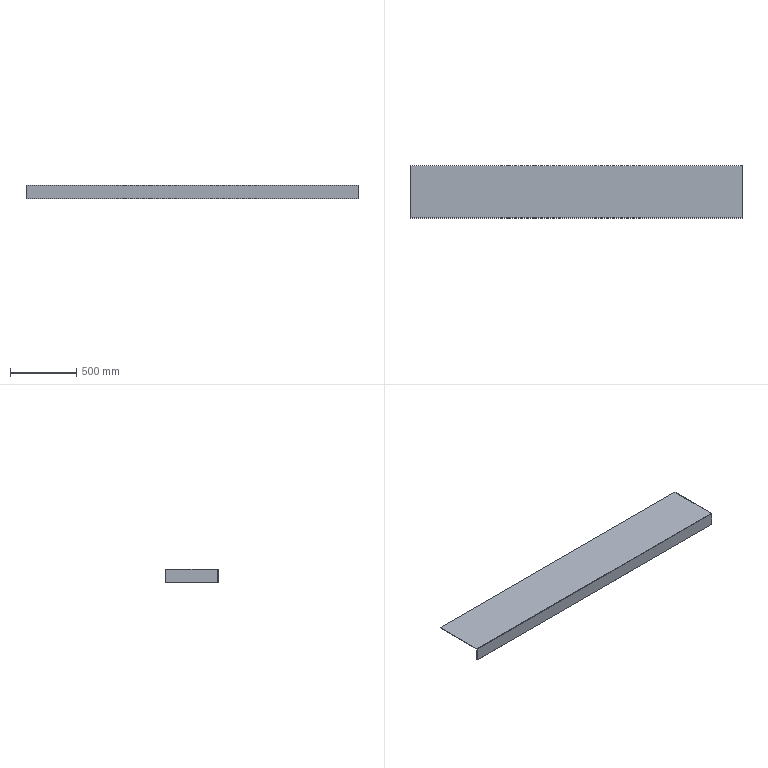Part | STEP file | PN_0035 third-floor site mounting plate 1_Default<As Machined> | 2 solids | 14 faces | box 2515 x 394 x 103 mm | volume 3844530 mm3 | plane 14
STEP:
#1=CARTESIAN_POINT('',(0.,0.,0.));
#2=DIRECTION('',(0.,0.,1.));
#3=DIRECTION('',(1.,0.,0.));
#4=AXIS2_PLACEMENT_3D('',#1,#2,#3);
#5=CARTESIAN_POINT('',(1257.5,-197.,0.));
#6=VERTEX_POINT('',#5);
#7=CARTESIAN_POINT('',(1257.5,197.,0.));
#8=VERTEX_POINT('',#7);
#9=CARTESIAN_POINT('',(1257.5,197.,0.));
#10=DIRECTION('',(0.,1.,0.));
#11=VECTOR('',#10,1.);
#12=LINE('',#9,#11);
#13=CARTESIAN_POINT('',(1257.5,197.,-3.));
#14=DIRECTION('',(1.,0.,0.));
#15=DIRECTION('',(0.,0.,-1.));
#16=AXIS2_PLACEMENT_3D('',#13,#14,#15);
#17=PLANE('',#16);
#18=CARTESIAN_POINT('',(-3.,0.));
#19=DIRECTION('',(0.,1.));
#20=VECTOR('',#19,1.);
#21=LINE('',#18,#20);
#22=(GEOMETRIC_REPRESENTATION_CONTEXT(2)PARAMETRIC_REPRESENTATION_CONTEXT()REPRESENTATION_CONTEXT('',''));
#23=DEFINITIONAL_REPRESENTATION('',(#21),#22);
#24=PCURVE('',#17,#23);
#25=CARTESIAN_POINT('',(0.,0.,0.));
#26=DIRECTION('',(0.,0.,1.));
#27=DIRECTION('',(1.,0.,0.));
#28=AXIS2_PLACEMENT_3D('',#25,#26,#27);
#29=PLANE('',#28);
#30=CARTESIAN_POINT('',(1257.5,197.));
#31=DIRECTION('',(0.,1.));
#32=VECTOR('',#31,1.);
#33=LINE('',#30,#32);
#34=(GEOMETRIC_REPRESENTATION_CONTEXT(2)PARAMETRIC_REPRESENTATION_CONTEXT()REPRESENTATION_CONTEXT('',''));
#35=DEFINITIONAL_REPRESENTATION('',(#33),#34);
#36=PCURVE('',#29,#35);
#37=SURFACE_CURVE('',#12,(#24,#36),.PCURVE_S1.);
#38=EDGE_CURVE('',#6,#8,#37,.T.);
#39=ORIENTED_EDGE('',*,*,#38,.F.);
#40=CARTESIAN_POINT('',(1257.5,-197.,-3.));
#41=VERTEX_POINT('',#40);
#42=CARTESIAN_POINT('',(1257.5,-197.,-3.));
#43=DIRECTION('',(0.,0.,1.));
#44=VECTOR('',#43,1.);
#45=LINE('',#42,#44);
#46=CARTESIAN_POINT('',(0.,-394.));
#47=DIRECTION('',(-1.,0.));
#48=VECTOR('',#47,1.);
#49=LINE('',#46,#48);
#50=(GEOMETRIC_REPRESENTATION_CONTEXT(2)PARAMETRIC_REPRESENTATION_CONTEXT()REPRESENTATION_CONTEXT('',''));
#51=DEFINITIONAL_REPRESENTATION('',(#49),#50);
#52=PCURVE('',#17,#51);
#53=CARTESIAN_POINT('',(-1257.5,-197.,-3.));
#54=DIRECTION('',(0.,-1.,0.));
#55=DIRECTION('',(0.,0.,-1.));
#56=AXIS2_PLACEMENT_3D('',#53,#54,#55);
#57=PLANE('',#56);
#58=CARTESIAN_POINT('',(0.,2515.));
#59=DIRECTION('',(-1.,0.));
#60=VECTOR('',#59,1.);
#61=LINE('',#58,#60);
#62=(GEOMETRIC_REPRESENTATION_CONTEXT(2)PARAMETRIC_REPRESENTATION_CONTEXT()REPRESENTATION_CONTEXT('',''));
#63=DEFINITIONAL_REPRESENTATION('',(#61),#62);
#64=PCURVE('',#57,#63);
#65=SURFACE_CURVE('',#45,(#52,#64),.PCURVE_S1.);
#66=EDGE_CURVE('',#41,#6,#65,.T.);
#67=ORIENTED_EDGE('',*,*,#66,.F.);
#68=CARTESIAN_POINT('',(1257.5,197.,-3.));
#69=VERTEX_POINT('',#68);
#70=CARTESIAN_POINT('',(1257.5,197.,-3.));
#71=DIRECTION('',(0.,1.,0.));
#72=VECTOR('',#71,1.);
#73=LINE('',#70,#72);
#74=CARTESIAN_POINT('',(0.,0.));
#75=DIRECTION('',(0.,1.));
#76=VECTOR('',#75,1.);
#77=LINE('',#74,#76);
#78=(GEOMETRIC_REPRESENTATION_CONTEXT(2)PARAMETRIC_REPRESENTATION_CONTEXT()REPRESENTATION_CONTEXT('',''));
#79=DEFINITIONAL_REPRESENTATION('',(#77),#78);
#80=PCURVE('',#17,#79);
#81=CARTESIAN_POINT('',(0.,0.,-3.));
#82=DIRECTION('',(0.,0.,1.));
#83=DIRECTION('',(1.,0.,0.));
#84=AXIS2_PLACEMENT_3D('',#81,#82,#83);
#85=PLANE('',#84);
#86=CARTESIAN_POINT('',(1257.5,197.));
#87=DIRECTION('',(0.,1.));
#88=VECTOR('',#87,1.);
#89=LINE('',#86,#88);
#90=(GEOMETRIC_REPRESENTATION_CONTEXT(2)PARAMETRIC_REPRESENTATION_CONTEXT()REPRESENTATION_CONTEXT('',''));
#91=DEFINITIONAL_REPRESENTATION('',(#89),#90);
#92=PCURVE('',#85,#91);
#93=SURFACE_CURVE('',#73,(#80,#92),.PCURVE_S1.);
#94=EDGE_CURVE('',#41,#69,#93,.T.);
#95=ORIENTED_EDGE('',*,*,#94,.T.);
#96=CARTESIAN_POINT('',(1257.5,197.,-3.));
#97=DIRECTION('',(0.,0.,1.));
#98=VECTOR('',#97,1.);
#99=LINE('',#96,#98);
#100=CARTESIAN_POINT('',(0.,0.));
#101=DIRECTION('',(-1.,0.));
#102=VECTOR('',#101,1.);
#103=LINE('',#100,#102);
#104=(GEOMETRIC_REPRESENTATION_CONTEXT(2)PARAMETRIC_REPRESENTATION_CONTEXT()REPRESENTATION_CONTEXT('',''));
#105=DEFINITIONAL_REPRESENTATION('',(#103),#104);
#106=PCURVE('',#17,#105);
#107=CARTESIAN_POINT('',(-1257.5,197.,-3.));
#108=DIRECTION('',(0.,1.,0.));
#109=DIRECTION('',(0.,0.,1.));
#110=AXIS2_PLACEMENT_3D('',#107,#108,#109);
#111=PLANE('',#110);
#112=CARTESIAN_POINT('',(0.,2515.));
#113=DIRECTION('',(1.,0.));
#114=VECTOR('',#113,1.);
#115=LINE('',#112,#114);
#116=(GEOMETRIC_REPRESENTATION_CONTEXT(2)PARAMETRIC_REPRESENTATION_CONTEXT()REPRESENTATION_CONTEXT('',''));
#117=DEFINITIONAL_REPRESENTATION('',(#115),#116);
#118=PCURVE('',#111,#117);
#119=SURFACE_CURVE('',#99,(#106,#118),.PCURVE_S1.);
#120=EDGE_CURVE('',#69,#8,#119,.T.);
#121=ORIENTED_EDGE('',*,*,#120,.T.);
#122=EDGE_LOOP('',(#39,#67,#95,#121));
#123=FACE_BOUND('',#122,.T.);
#124=ADVANCED_FACE('',(#123),#17,.T.);
#125=CARTESIAN_POINT('',(-1257.5,-197.,0.));
#126=VERTEX_POINT('',#125);
#127=CARTESIAN_POINT('',(-1257.5,-197.,0.));
#128=DIRECTION('',(1.,0.,0.));
#129=VECTOR('',#128,1.);
#130=LINE('',#127,#129);
#131=CARTESIAN_POINT('',(-3.,0.));
#132=DIRECTION('',(0.,1.));
#133=VECTOR('',#132,1.);
#134=LINE('',#131,#133);
#135=(GEOMETRIC_REPRESENTATION_CONTEXT(2)PARAMETRIC_REPRESENTATION_CONTEXT()REPRESENTATION_CONTEXT('',''));
#136=DEFINITIONAL_REPRESENTATION('',(#134),#135);
#137=PCURVE('',#57,#136);
#138=CARTESIAN_POINT('',(-1257.5,-197.));
#139=DIRECTION('',(1.,0.));
#140=VECTOR('',#139,1.);
#141=LINE('',#138,#140);
#142=(GEOMETRIC_REPRESENTATION_CONTEXT(2)PARAMETRIC_REPRESENTATION_CONTEXT()REPRESENTATION_CONTEXT('',''));
#143=DEFINITIONAL_REPRESENTATION('',(#141),#142);
#144=PCURVE('',#29,#143);
#145=SURFACE_CURVE('',#130,(#137,#144),.PCURVE_S1.);
#146=EDGE_CURVE('',#126,#6,#145,.T.);
#147=ORIENTED_EDGE('',*,*,#146,.F.);
#148=CARTESIAN_POINT('',(-1257.5,-197.,-3.));
#149=VERTEX_POINT('',#148);
#150=CARTESIAN_POINT('',(-1257.5,-197.,-3.));
#151=DIRECTION('',(0.,0.,1.));
#152=VECTOR('',#151,1.);
#153=LINE('',#150,#152);
#154=CARTESIAN_POINT('',(0.,0.));
#155=DIRECTION('',(-1.,0.));
#156=VECTOR('',#155,1.);
#157=LINE('',#154,#156);
#158=(GEOMETRIC_REPRESENTATION_CONTEXT(2)PARAMETRIC_REPRESENTATION_CONTEXT()REPRESENTATION_CONTEXT('',''));
#159=DEFINITIONAL_REPRESENTATION('',(#157),#158);
#160=PCURVE('',#57,#159);
#161=CARTESIAN_POINT('',(-1257.5,197.,-3.));
#162=DIRECTION('',(-1.,0.,0.));
#163=DIRECTION('',(0.,0.,1.));
#164=AXIS2_PLACEMENT_3D('',#161,#162,#163);
#165=PLANE('',#164);
#166=CARTESIAN_POINT('',(0.,-394.));
#167=DIRECTION('',(1.,0.));
#168=VECTOR('',#167,1.);
#169=LINE('',#166,#168);
#170=(GEOMETRIC_REPRESENTATION_CONTEXT(2)PARAMETRIC_REPRESENTATION_CONTEXT()REPRESENTATION_CONTEXT('',''));
#171=DEFINITIONAL_REPRESENTATION('',(#169),#170);
#172=PCURVE('',#165,#171);
#173=SURFACE_CURVE('',#153,(#160,#172),.PCURVE_S1.);
#174=EDGE_CURVE('',#149,#126,#173,.T.);
#175=ORIENTED_EDGE('',*,*,#174,.F.);
#176=CARTESIAN_POINT('',(-1257.5,-197.,-3.));
#177=DIRECTION('',(1.,0.,0.));
#178=VECTOR('',#177,1.);
#179=LINE('',#176,#178);
#180=CARTESIAN_POINT('',(0.,0.));
#181=DIRECTION('',(0.,1.));
#182=VECTOR('',#181,1.);
#183=LINE('',#180,#182);
#184=(GEOMETRIC_REPRESENTATION_CONTEXT(2)PARAMETRIC_REPRESENTATION_CONTEXT()REPRESENTATION_CONTEXT('',''));
#185=DEFINITIONAL_REPRESENTATION('',(#183),#184);
#186=PCURVE('',#57,#185);
#187=CARTESIAN_POINT('',(-1257.5,-197.));
#188=DIRECTION('',(1.,0.));
#189=VECTOR('',#188,1.);
#190=LINE('',#187,#189);
#191=(GEOMETRIC_REPRESENTATION_CONTEXT(2)PARAMETRIC_REPRESENTATION_CONTEXT()REPRESENTATION_CONTEXT('',''));
#192=DEFINITIONAL_REPRESENTATION('',(#190),#191);
#193=PCURVE('',#85,#192);
#194=SURFACE_CURVE('',#179,(#186,#193),.PCURVE_S1.);
#195=EDGE_CURVE('',#149,#41,#194,.T.);
#196=ORIENTED_EDGE('',*,*,#195,.T.);
#197=ORIENTED_EDGE('',*,*,#66,.T.);
#198=EDGE_LOOP('',(#147,#175,#196,#197));
#199=FACE_BOUND('',#198,.T.);
#200=ADVANCED_FACE('',(#199),#57,.T.);
#201=CARTESIAN_POINT('',(-1257.5,197.,0.));
#202=VERTEX_POINT('',#201);
#203=CARTESIAN_POINT('',(-1257.5,197.,0.));
#204=DIRECTION('',(0.,-1.,0.));
#205=VECTOR('',#204,1.);
#206=LINE('',#203,#205);
#207=CARTESIAN_POINT('',(3.,0.));
#208=DIRECTION('',(0.,-1.));
#209=VECTOR('',#208,1.);
#210=LINE('',#207,#209);
#211=(GEOMETRIC_REPRESENTATION_CONTEXT(2)PARAMETRIC_REPRESENTATION_CONTEXT()REPRESENTATION_CONTEXT('',''));
#212=DEFINITIONAL_REPRESENTATION('',(#210),#211);
#213=PCURVE('',#165,#212);
#214=CARTESIAN_POINT('',(-1257.5,197.));
#215=DIRECTION('',(0.,-1.));
#216=VECTOR('',#215,1.);
#217=LINE('',#214,#216);
#218=(GEOMETRIC_REPRESENTATION_CONTEXT(2)PARAMETRIC_REPRESENTATION_CONTEXT()REPRESENTATION_CONTEXT('',''));
#219=DEFINITIONAL_REPRESENTATION('',(#217),#218);
#220=PCURVE('',#29,#219);
#221=SURFACE_CURVE('',#206,(#213,#220),.PCURVE_S1.);
#222=EDGE_CURVE('',#202,#126,#221,.T.);
#223=ORIENTED_EDGE('',*,*,#222,.F.);
#224=CARTESIAN_POINT('',(-1257.5,197.,-3.));
#225=VERTEX_POINT('',#224);
#226=CARTESIAN_POINT('',(-1257.5,197.,-3.));
#227=DIRECTION('',(0.,0.,1.));
#228=VECTOR('',#227,1.);
#229=LINE('',#226,#228);
#230=CARTESIAN_POINT('',(0.,0.));
#231=DIRECTION('',(1.,0.));
#232=VECTOR('',#231,1.);
#233=LINE('',#230,#232);
#234=(GEOMETRIC_REPRESENTATION_CONTEXT(2)PARAMETRIC_REPRESENTATION_CONTEXT()REPRESENTATION_CONTEXT('',''));
#235=DEFINITIONAL_REPRESENTATION('',(#233),#234);
#236=PCURVE('',#165,#235);
#237=CARTESIAN_POINT('',(0.,0.));
#238=DIRECTION('',(1.,0.));
#239=VECTOR('',#238,1.);
#240=LINE('',#237,#239);
#241=(GEOMETRIC_REPRESENTATION_CONTEXT(2)PARAMETRIC_REPRESENTATION_CONTEXT()REPRESENTATION_CONTEXT('',''));
#242=DEFINITIONAL_REPRESENTATION('',(#240),#241);
#243=PCURVE('',#111,#242);
#244=SURFACE_CURVE('',#229,(#236,#243),.PCURVE_S1.);
#245=EDGE_CURVE('',#225,#202,#244,.T.);
#246=ORIENTED_EDGE('',*,*,#245,.F.);
#247=CARTESIAN_POINT('',(-1257.5,197.,-3.));
#248=DIRECTION('',(0.,-1.,0.));
#249=VECTOR('',#248,1.);
#250=LINE('',#247,#249);
#251=CARTESIAN_POINT('',(0.,0.));
#252=DIRECTION('',(0.,-1.));
#253=VECTOR('',#252,1.);
#254=LINE('',#251,#253);
#255=(GEOMETRIC_REPRESENTATION_CONTEXT(2)PARAMETRIC_REPRESENTATION_CONTEXT()REPRESENTATION_CONTEXT('',''));
#256=DEFINITIONAL_REPRESENTATION('',(#254),#255);
#257=PCURVE('',#165,#256);
#258=CARTESIAN_POINT('',(-1257.5,197.));
#259=DIRECTION('',(0.,-1.));
#260=VECTOR('',#259,1.);
#261=LINE('',#258,#260);
#262=(GEOMETRIC_REPRESENTATION_CONTEXT(2)PARAMETRIC_REPRESENTATION_CONTEXT()REPRESENTATION_CONTEXT('',''));
#263=DEFINITIONAL_REPRESENTATION('',(#261),#262);
#264=PCURVE('',#85,#263);
#265=SURFACE_CURVE('',#250,(#257,#264),.PCURVE_S1.);
#266=EDGE_CURVE('',#225,#149,#265,.T.);
#267=ORIENTED_EDGE('',*,*,#266,.T.);
#268=ORIENTED_EDGE('',*,*,#174,.T.);
#269=EDGE_LOOP('',(#223,#246,#267,#268));
#270=FACE_BOUND('',#269,.T.);
#271=ADVANCED_FACE('',(#270),#165,.T.);
#272=CARTESIAN_POINT('',(-1257.5,197.,0.));
#273=DIRECTION('',(-1.,0.,0.));
#274=VECTOR('',#273,1.);
#275=LINE('',#272,#274);
#276=CARTESIAN_POINT('',(3.,0.));
#277=DIRECTION('',(0.,-1.));
#278=VECTOR('',#277,1.);
#279=LINE('',#276,#278);
#280=(GEOMETRIC_REPRESENTATION_CONTEXT(2)PARAMETRIC_REPRESENTATION_CONTEXT()REPRESENTATION_CONTEXT('',''));
#281=DEFINITIONAL_REPRESENTATION('',(#279),#280);
#282=PCURVE('',#111,#281);
#283=CARTESIAN_POINT('',(-1257.5,197.));
#284=DIRECTION('',(-1.,0.));
#285=VECTOR('',#284,1.);
#286=LINE('',#283,#285);
#287=(GEOMETRIC_REPRESENTATION_CONTEXT(2)PARAMETRIC_REPRESENTATION_CONTEXT()REPRESENTATION_CONTEXT('',''));
#288=DEFINITIONAL_REPRESENTATION('',(#286),#287);
#289=PCURVE('',#29,#288);
#290=SURFACE_CURVE('',#275,(#282,#289),.PCURVE_S1.);
#291=EDGE_CURVE('',#8,#202,#290,.T.);
#292=ORIENTED_EDGE('',*,*,#291,.F.);
#293=ORIENTED_EDGE('',*,*,#120,.F.);
#294=CARTESIAN_POINT('',(-1257.5,197.,-3.));
#295=DIRECTION('',(-1.,0.,0.));
#296=VECTOR('',#295,1.);
#297=LINE('',#294,#296);
#298=CARTESIAN_POINT('',(0.,0.));
#299=DIRECTION('',(0.,-1.));
#300=VECTOR('',#299,1.);
#301=LINE('',#298,#300);
#302=(GEOMETRIC_REPRESENTATION_CONTEXT(2)PARAMETRIC_REPRESENTATION_CONTEXT()REPRESENTATION_CONTEXT('',''));
#303=DEFINITIONAL_REPRESENTATION('',(#301),#302);
#304=PCURVE('',#111,#303);
#305=CARTESIAN_POINT('',(-1257.5,197.));
#306=DIRECTION('',(-1.,0.));
#307=VECTOR('',#306,1.);
#308=LINE('',#305,#307);
#309=(GEOMETRIC_REPRESENTATION_CONTEXT(2)PARAMETRIC_REPRESENTATION_CONTEXT()REPRESENTATION_CONTEXT('',''));
#310=DEFINITIONAL_REPRESENTATION('',(#308),#309);
#311=PCURVE('',#85,#310);
#312=SURFACE_CURVE('',#297,(#304,#311),.PCURVE_S1.);
#313=EDGE_CURVE('',#69,#225,#312,.T.);
#314=ORIENTED_EDGE('',*,*,#313,.T.);
#315=ORIENTED_EDGE('',*,*,#245,.T.);
#316=EDGE_LOOP('',(#292,#293,#314,#315));
#317=FACE_BOUND('',#316,.T.);
#318=ADVANCED_FACE('',(#317),#111,.T.);
#319=ORIENTED_EDGE('',*,*,#94,.F.);
#320=ORIENTED_EDGE('',*,*,#195,.F.);
#321=ORIENTED_EDGE('',*,*,#266,.F.);
#322=ORIENTED_EDGE('',*,*,#313,.F.);
#323=EDGE_LOOP('',(#319,#320,#321,#322));
#324=FACE_BOUND('',#323,.T.);
#325=ADVANCED_FACE('',(#324),#85,.F.);
#326=ORIENTED_EDGE('',*,*,#38,.T.);
#327=ORIENTED_EDGE('',*,*,#291,.T.);
#328=ORIENTED_EDGE('',*,*,#222,.T.);
#329=ORIENTED_EDGE('',*,*,#146,.T.);
#330=EDGE_LOOP('',(#326,#327,#328,#329));
#331=FACE_BOUND('',#330,.T.);
#332=ADVANCED_FACE('',(#331),#29,.T.);
#333=CLOSED_SHELL('',(#124,#200,#271,#318,#325,#332));
#334=MANIFOLD_SOLID_BREP('',#333);
#335=CARTESIAN_POINT('',(1254.5,-194.,-3.));
#336=VERTEX_POINT('',#335);
#337=CARTESIAN_POINT('',(1254.5,197.,-3.));
#338=VERTEX_POINT('',#337);
#339=CARTESIAN_POINT('',(1254.5,-197.,-3.));
#340=DIRECTION('',(0.,1.,0.));
#341=VECTOR('',#340,1.);
#342=LINE('',#339,#341);
#343=CARTESIAN_POINT('',(1254.5,-197.,-103.));
#344=DIRECTION('',(1.,0.,0.));
#345=DIRECTION('',(0.,0.,-1.));
#346=AXIS2_PLACEMENT_3D('',#343,#344,#345);
#347=PLANE('',#346);
#348=CARTESIAN_POINT('',(-100.,0.));
#349=DIRECTION('',(0.,1.));
#350=VECTOR('',#349,1.);
#351=LINE('',#348,#350);
#352=(GEOMETRIC_REPRESENTATION_CONTEXT(2)PARAMETRIC_REPRESENTATION_CONTEXT()REPRESENTATION_CONTEXT('',''));
#353=DEFINITIONAL_REPRESENTATION('',(#351),#352);
#354=PCURVE('',#347,#353);
#355=CARTESIAN_POINT('',(0.,0.,-3.));
#356=DIRECTION('',(0.,0.,1.));
#357=DIRECTION('',(1.,0.,0.));
#358=AXIS2_PLACEMENT_3D('',#355,#356,#357);
#359=PLANE('',#358);
#360=CARTESIAN_POINT('',(1254.5,-197.));
#361=DIRECTION('',(0.,1.));
#362=VECTOR('',#361,1.);
#363=LINE('',#360,#362);
#364=(GEOMETRIC_REPRESENTATION_CONTEXT(2)PARAMETRIC_REPRESENTATION_CONTEXT()REPRESENTATION_CONTEXT('',''));
#365=DEFINITIONAL_REPRESENTATION('',(#363),#364);
#366=PCURVE('',#359,#365);
#367=SURFACE_CURVE('',#342,(#354,#366),.PCURVE_S1.);
#368=EDGE_CURVE('',#336,#338,#367,.T.);
#369=ORIENTED_EDGE('',*,*,#368,.T.);
#370=CARTESIAN_POINT('',(1254.5,197.,-103.));
#371=VERTEX_POINT('',#370);
#372=CARTESIAN_POINT('',(1254.5,197.,-103.));
#373=DIRECTION('',(0.,0.,1.));
#374=VECTOR('',#373,1.);
#375=LINE('',#372,#374);
#376=CARTESIAN_POINT('',(0.,394.));
#377=DIRECTION('',(-1.,0.));
#378=VECTOR('',#377,1.);
#379=LINE('',#376,#378);
#380=(GEOMETRIC_REPRESENTATION_CONTEXT(2)PARAMETRIC_REPRESENTATION_CONTEXT()REPRESENTATION_CONTEXT('',''));
#381=DEFINITIONAL_REPRESENTATION('',(#379),#380);
#382=PCURVE('',#347,#381);
#383=CARTESIAN_POINT('',(1257.5,197.,-103.));
#384=DIRECTION('',(0.,1.,0.));
#385=DIRECTION('',(0.,0.,1.));
#386=AXIS2_PLACEMENT_3D('',#383,#384,#385);
#387=PLANE('',#386);
#388=CARTESIAN_POINT('',(0.,-3.));
#389=DIRECTION('',(1.,0.));
#390=VECTOR('',#389,1.);
#391=LINE('',#388,#390);
#392=(GEOMETRIC_REPRESENTATION_CONTEXT(2)PARAMETRIC_REPRESENTATION_CONTEXT()REPRESENTATION_CONTEXT('',''));
#393=DEFINITIONAL_REPRESENTATION('',(#391),#392);
#394=PCURVE('',#387,#393);
#395=SURFACE_CURVE('',#375,(#382,#394),.PCURVE_S1.);
#396=EDGE_CURVE('',#371,#338,#395,.T.);
#397=ORIENTED_EDGE('',*,*,#396,.F.);
#398=CARTESIAN_POINT('',(1254.5,-194.,-103.));
#399=VERTEX_POINT('',#398);
#400=CARTESIAN_POINT('',(1254.5,-197.,-103.));
#401=DIRECTION('',(0.,1.,0.));
#402=VECTOR('',#401,1.);
#403=LINE('',#400,#402);
#404=CARTESIAN_POINT('',(0.,0.));
#405=DIRECTION('',(0.,1.));
#406=VECTOR('',#405,1.);
#407=LINE('',#404,#406);
#408=(GEOMETRIC_REPRESENTATION_CONTEXT(2)PARAMETRIC_REPRESENTATION_CONTEXT()REPRESENTATION_CONTEXT('',''));
#409=DEFINITIONAL_REPRESENTATION('',(#407),#408);
#410=PCURVE('',#347,#409);
#411=CARTESIAN_POINT('',(0.,0.,-103.));
#412=DIRECTION('',(0.,0.,1.));
#413=DIRECTION('',(1.,0.,0.));
#414=AXIS2_PLACEMENT_3D('',#411,#412,#413);
#415=PLANE('',#414);
#416=CARTESIAN_POINT('',(1254.5,-197.));
#417=DIRECTION('',(0.,1.));
#418=VECTOR('',#417,1.);
#419=LINE('',#416,#418);
#420=(GEOMETRIC_REPRESENTATION_CONTEXT(2)PARAMETRIC_REPRESENTATION_CONTEXT()REPRESENTATION_CONTEXT('',''));
#421=DEFINITIONAL_REPRESENTATION('',(#419),#420);
#422=PCURVE('',#415,#421);
#423=SURFACE_CURVE('',#403,(#410,#422),.PCURVE_S1.);
#424=EDGE_CURVE('',#399,#371,#423,.T.);
#425=ORIENTED_EDGE('',*,*,#424,.F.);
#426=CARTESIAN_POINT('',(1254.5,-194.,-103.));
#427=DIRECTION('',(0.,0.,1.));
#428=VECTOR('',#427,1.);
#429=LINE('',#426,#428);
#430=CARTESIAN_POINT('',(0.,3.));
#431=DIRECTION('',(-1.,0.));
#432=VECTOR('',#431,1.);
#433=LINE('',#430,#432);
#434=(GEOMETRIC_REPRESENTATION_CONTEXT(2)PARAMETRIC_REPRESENTATION_CONTEXT()REPRESENTATION_CONTEXT('',''));
#435=DEFINITIONAL_REPRESENTATION('',(#433),#434);
#436=PCURVE('',#347,#435);
#437=CARTESIAN_POINT('',(-1257.5,-194.,-103.));
#438=DIRECTION('',(0.,-1.,0.));
#439=DIRECTION('',(0.,0.,-1.));
#440=AXIS2_PLACEMENT_3D('',#437,#438,#439);
#441=PLANE('',#440);
#442=CARTESIAN_POINT('',(0.,2512.));
#443=DIRECTION('',(-1.,0.));
#444=VECTOR('',#443,1.);
#445=LINE('',#442,#444);
#446=(GEOMETRIC_REPRESENTATION_CONTEXT(2)PARAMETRIC_REPRESENTATION_CONTEXT()REPRESENTATION_CONTEXT('',''));
#447=DEFINITIONAL_REPRESENTATION('',(#445),#446);
#448=PCURVE('',#441,#447);
#449=SURFACE_CURVE('',#429,(#436,#448),.PCURVE_S1.);
#450=EDGE_CURVE('',#399,#336,#449,.T.);
#451=ORIENTED_EDGE('',*,*,#450,.T.);
#452=EDGE_LOOP('',(#369,#397,#425,#451));
#453=FACE_BOUND('',#452,.T.);
#454=ADVANCED_FACE('',(#453),#347,.F.);
#455=CARTESIAN_POINT('',(1257.5,197.,-3.));
#456=VERTEX_POINT('',#455);
#457=CARTESIAN_POINT('',(1257.5,197.,-3.));
#458=DIRECTION('',(-1.,0.,0.));
#459=VECTOR('',#458,1.);
#460=LINE('',#457,#459);
#461=CARTESIAN_POINT('',(100.,0.));
#462=DIRECTION('',(0.,-1.));
#463=VECTOR('',#462,1.);
#464=LINE('',#461,#463);
#465=(GEOMETRIC_REPRESENTATION_CONTEXT(2)PARAMETRIC_REPRESENTATION_CONTEXT()REPRESENTATION_CONTEXT('',''));
#466=DEFINITIONAL_REPRESENTATION('',(#464),#465);
#467=PCURVE('',#387,#466);
#468=CARTESIAN_POINT('',(1257.5,197.));
#469=DIRECTION('',(-1.,0.));
#470=VECTOR('',#469,1.);
#471=LINE('',#468,#470);
#472=(GEOMETRIC_REPRESENTATION_CONTEXT(2)PARAMETRIC_REPRESENTATION_CONTEXT()REPRESENTATION_CONTEXT('',''));
#473=DEFINITIONAL_REPRESENTATION('',(#471),#472);
#474=PCURVE('',#359,#473);
#475=SURFACE_CURVE('',#460,(#467,#474),.PCURVE_S1.);
#476=EDGE_CURVE('',#456,#338,#475,.T.);
#477=ORIENTED_EDGE('',*,*,#476,.F.);
#478=CARTESIAN_POINT('',(1257.5,197.,-103.));
#479=VERTEX_POINT('',#478);
#480=CARTESIAN_POINT('',(1257.5,197.,-103.));
#481=DIRECTION('',(0.,0.,1.));
#482=VECTOR('',#481,1.);
#483=LINE('',#480,#482);
#484=CARTESIAN_POINT('',(0.,0.));
#485=DIRECTION('',(1.,0.));
#486=VECTOR('',#485,1.);
#487=LINE('',#484,#486);
#488=(GEOMETRIC_REPRESENTATION_CONTEXT(2)PARAMETRIC_REPRESENTATION_CONTEXT()REPRESENTATION_CONTEXT('',''));
#489=DEFINITIONAL_REPRESENTATION('',(#487),#488);
#490=PCURVE('',#387,#489);
#491=CARTESIAN_POINT('',(1257.5,-197.,-103.));
#492=DIRECTION('',(1.,0.,0.));
#493=DIRECTION('',(0.,0.,-1.));
#494=AXIS2_PLACEMENT_3D('',#491,#492,#493);
#495=PLANE('',#494);
#496=CARTESIAN_POINT('',(0.,394.));
#497=DIRECTION('',(-1.,0.));
#498=VECTOR('',#497,1.);
#499=LINE('',#496,#498);
#500=(GEOMETRIC_REPRESENTATION_CONTEXT(2)PARAMETRIC_REPRESENTATION_CONTEXT()REPRESENTATION_CONTEXT('',''));
#501=DEFINITIONAL_REPRESENTATION('',(#499),#500);
#502=PCURVE('',#495,#501);
#503=SURFACE_CURVE('',#483,(#490,#502),.PCURVE_S1.);
#504=EDGE_CURVE('',#479,#456,#503,.T.);
#505=ORIENTED_EDGE('',*,*,#504,.F.);
#506=CARTESIAN_POINT('',(1257.5,197.,-103.));
#507=DIRECTION('',(-1.,0.,0.));
#508=VECTOR('',#507,1.);
#509=LINE('',#506,#508);
#510=CARTESIAN_POINT('',(0.,0.));
#511=DIRECTION('',(0.,-1.));
#512=VECTOR('',#511,1.);
#513=LINE('',#510,#512);
#514=(GEOMETRIC_REPRESENTATION_CONTEXT(2)PARAMETRIC_REPRESENTATION_CONTEXT()REPRESENTATION_CONTEXT('',''));
#515=DEFINITIONAL_REPRESENTATION('',(#513),#514);
#516=PCURVE('',#387,#515);
#517=CARTESIAN_POINT('',(1257.5,197.));
#518=DIRECTION('',(-1.,0.));
#519=VECTOR('',#518,1.);
#520=LINE('',#517,#519);
#521=(GEOMETRIC_REPRESENTATION_CONTEXT(2)PARAMETRIC_REPRESENTATION_CONTEXT()REPRESENTATION_CONTEXT('',''));
#522=DEFINITIONAL_REPRESENTATION('',(#520),#521);
#523=PCURVE('',#415,#522);
#524=SURFACE_CURVE('',#509,(#516,#523),.PCURVE_S1.);
#525=EDGE_CURVE('',#479,#371,#524,.T.);
#526=ORIENTED_EDGE('',*,*,#525,.T.);
#527=ORIENTED_EDGE('',*,*,#396,.T.);
#528=EDGE_LOOP('',(#477,#505,#526,#527));
#529=FACE_BOUND('',#528,.T.);
#530=ADVANCED_FACE('',(#529),#387,.T.);
#531=CARTESIAN_POINT('',(1257.5,-197.,-3.));
#532=VERTEX_POINT('',#531);
#533=CARTESIAN_POINT('',(1257.5,-197.,-3.));
#534=DIRECTION('',(0.,1.,0.));
#535=VECTOR('',#534,1.);
#536=LINE('',#533,#535);
#537=CARTESIAN_POINT('',(-100.,0.));
#538=DIRECTION('',(0.,1.));
#539=VECTOR('',#538,1.);
#540=LINE('',#537,#539);
#541=(GEOMETRIC_REPRESENTATION_CONTEXT(2)PARAMETRIC_REPRESENTATION_CONTEXT()REPRESENTATION_CONTEXT('',''));
#542=DEFINITIONAL_REPRESENTATION('',(#540),#541);
#543=PCURVE('',#495,#542);
#544=CARTESIAN_POINT('',(1257.5,-197.));
#545=DIRECTION('',(0.,1.));
#546=VECTOR('',#545,1.);
#547=LINE('',#544,#546);
#548=(GEOMETRIC_REPRESENTATION_CONTEXT(2)PARAMETRIC_REPRESENTATION_CONTEXT()REPRESENTATION_CONTEXT('',''));
#549=DEFINITIONAL_REPRESENTATION('',(#547),#548);
#550=PCURVE('',#359,#549);
#551=SURFACE_CURVE('',#536,(#543,#550),.PCURVE_S1.);
#552=EDGE_CURVE('',#532,#456,#551,.T.);
#553=ORIENTED_EDGE('',*,*,#552,.F.);
#554=CARTESIAN_POINT('',(1257.5,-197.,-103.));
#555=VERTEX_POINT('',#554);
#556=CARTESIAN_POINT('',(1257.5,-197.,-103.));
#557=DIRECTION('',(0.,0.,1.));
#558=VECTOR('',#557,1.);
#559=LINE('',#556,#558);
#560=CARTESIAN_POINT('',(0.,0.));
#561=DIRECTION('',(-1.,0.));
#562=VECTOR('',#561,1.);
#563=LINE('',#560,#562);
#564=(GEOMETRIC_REPRESENTATION_CONTEXT(2)PARAMETRIC_REPRESENTATION_CONTEXT()REPRESENTATION_CONTEXT('',''));
#565=DEFINITIONAL_REPRESENTATION('',(#563),#564);
#566=PCURVE('',#495,#565);
#567=CARTESIAN_POINT('',(-1257.5,-197.,-103.));
#568=DIRECTION('',(0.,-1.,0.));
#569=DIRECTION('',(0.,0.,-1.));
#570=AXIS2_PLACEMENT_3D('',#567,#568,#569);
#571=PLANE('',#570);
#572=CARTESIAN_POINT('',(0.,2515.));
#573=DIRECTION('',(-1.,0.));
#574=VECTOR('',#573,1.);
#575=LINE('',#572,#574);
#576=(GEOMETRIC_REPRESENTATION_CONTEXT(2)PARAMETRIC_REPRESENTATION_CONTEXT()REPRESENTATION_CONTEXT('',''));
#577=DEFINITIONAL_REPRESENTATION('',(#575),#576);
#578=PCURVE('',#571,#577);
#579=SURFACE_CURVE('',#559,(#566,#578),.PCURVE_S1.);
#580=EDGE_CURVE('',#555,#532,#579,.T.);
#581=ORIENTED_EDGE('',*,*,#580,.F.);
#582=CARTESIAN_POINT('',(1257.5,-197.,-103.));
#583=DIRECTION('',(0.,1.,0.));
#584=VECTOR('',#583,1.);
#585=LINE('',#582,#584);
#586=CARTESIAN_POINT('',(0.,0.));
#587=DIRECTION('',(0.,1.));
#588=VECTOR('',#587,1.);
#589=LINE('',#586,#588);
#590=(GEOMETRIC_REPRESENTATION_CONTEXT(2)PARAMETRIC_REPRESENTATION_CONTEXT()REPRESENTATION_CONTEXT('',''));
#591=DEFINITIONAL_REPRESENTATION('',(#589),#590);
#592=PCURVE('',#495,#591);
#593=CARTESIAN_POINT('',(1257.5,-197.));
#594=DIRECTION('',(0.,1.));
#595=VECTOR('',#594,1.);
#596=LINE('',#593,#595);
#597=(GEOMETRIC_REPRESENTATION_CONTEXT(2)PARAMETRIC_REPRESENTATION_CONTEXT()REPRESENTATION_CONTEXT('',''));
#598=DEFINITIONAL_REPRESENTATION('',(#596),#597);
#599=PCURVE('',#415,#598);
#600=SURFACE_CURVE('',#585,(#592,#599),.PCURVE_S1.);
#601=EDGE_CURVE('',#555,#479,#600,.T.);
#602=ORIENTED_EDGE('',*,*,#601,.T.);
#603=ORIENTED_EDGE('',*,*,#504,.T.);
#604=EDGE_LOOP('',(#553,#581,#602,#603));
#605=FACE_BOUND('',#604,.T.);
#606=ADVANCED_FACE('',(#605),#495,.T.);
#607=CARTESIAN_POINT('',(-1257.5,-197.,-3.));
#608=VERTEX_POINT('',#607);
#609=CARTESIAN_POINT('',(-1257.5,-197.,-3.));
#610=DIRECTION('',(1.,0.,0.));
#611=VECTOR('',#610,1.);
#612=LINE('',#609,#611);
#613=CARTESIAN_POINT('',(-100.,0.));
#614=DIRECTION('',(0.,1.));
#615=VECTOR('',#614,1.);
#616=LINE('',#613,#615);
#617=(GEOMETRIC_REPRESENTATION_CONTEXT(2)PARAMETRIC_REPRESENTATION_CONTEXT()REPRESENTATION_CONTEXT('',''));
#618=DEFINITIONAL_REPRESENTATION('',(#616),#617);
#619=PCURVE('',#571,#618);
#620=CARTESIAN_POINT('',(-1257.5,-197.));
#621=DIRECTION('',(1.,0.));
#622=VECTOR('',#621,1.);
#623=LINE('',#620,#622);
#624=(GEOMETRIC_REPRESENTATION_CONTEXT(2)PARAMETRIC_REPRESENTATION_CONTEXT()REPRESENTATION_CONTEXT('',''));
#625=DEFINITIONAL_REPRESENTATION('',(#623),#624);
#626=PCURVE('',#359,#625);
#627=SURFACE_CURVE('',#612,(#619,#626),.PCURVE_S1.);
#628=EDGE_CURVE('',#608,#532,#627,.T.);
#629=ORIENTED_EDGE('',*,*,#628,.F.);
#630=CARTESIAN_POINT('',(-1257.5,-197.,-103.));
#631=VERTEX_POINT('',#630);
#632=CARTESIAN_POINT('',(-1257.5,-197.,-103.));
#633=DIRECTION('',(0.,0.,1.));
#634=VECTOR('',#633,1.);
#635=LINE('',#632,#634);
#636=CARTESIAN_POINT('',(0.,0.));
#637=DIRECTION('',(-1.,0.));
#638=VECTOR('',#637,1.);
#639=LINE('',#636,#638);
#640=(GEOMETRIC_REPRESENTATION_CONTEXT(2)PARAMETRIC_REPRESENTATION_CONTEXT()REPRESENTATION_CONTEXT('',''));
#641=DEFINITIONAL_REPRESENTATION('',(#639),#640);
#642=PCURVE('',#571,#641);
#643=CARTESIAN_POINT('',(-1257.5,-194.,-103.));
#644=DIRECTION('',(-1.,0.,0.));
#645=DIRECTION('',(0.,0.,1.));
#646=AXIS2_PLACEMENT_3D('',#643,#644,#645);
#647=PLANE('',#646);
#648=CARTESIAN_POINT('',(0.,-3.));
#649=DIRECTION('',(1.,0.));
#650=VECTOR('',#649,1.);
#651=LINE('',#648,#650);
#652=(GEOMETRIC_REPRESENTATION_CONTEXT(2)PARAMETRIC_REPRESENTATION_CONTEXT()REPRESENTATION_CONTEXT('',''));
#653=DEFINITIONAL_REPRESENTATION('',(#651),#652);
#654=PCURVE('',#647,#653);
#655=SURFACE_CURVE('',#635,(#642,#654),.PCURVE_S1.);
#656=EDGE_CURVE('',#631,#608,#655,.T.);
#657=ORIENTED_EDGE('',*,*,#656,.F.);
#658=CARTESIAN_POINT('',(-1257.5,-197.,-103.));
#659=DIRECTION('',(1.,0.,0.));
#660=VECTOR('',#659,1.);
#661=LINE('',#658,#660);
#662=CARTESIAN_POINT('',(0.,0.));
#663=DIRECTION('',(0.,1.));
#664=VECTOR('',#663,1.);
#665=LINE('',#662,#664);
#666=(GEOMETRIC_REPRESENTATION_CONTEXT(2)PARAMETRIC_REPRESENTATION_CONTEXT()REPRESENTATION_CONTEXT('',''));
#667=DEFINITIONAL_REPRESENTATION('',(#665),#666);
#668=PCURVE('',#571,#667);
#669=CARTESIAN_POINT('',(-1257.5,-197.));
#670=DIRECTION('',(1.,0.));
#671=VECTOR('',#670,1.);
#672=LINE('',#669,#671);
#673=(GEOMETRIC_REPRESENTATION_CONTEXT(2)PARAMETRIC_REPRESENTATION_CONTEXT()REPRESENTATION_CONTEXT('',''));
#674=DEFINITIONAL_REPRESENTATION('',(#672),#673);
#675=PCURVE('',#415,#674);
#676=SURFACE_CURVE('',#661,(#668,#675),.PCURVE_S1.);
#677=EDGE_CURVE('',#631,#555,#676,.T.);
#678=ORIENTED_EDGE('',*,*,#677,.T.);
#679=ORIENTED_EDGE('',*,*,#580,.T.);
#680=EDGE_LOOP('',(#629,#657,#678,#679));
#681=FACE_BOUND('',#680,.T.);
#682=ADVANCED_FACE('',(#681),#571,.T.);
#683=CARTESIAN_POINT('',(-1257.5,-194.,-3.));
#684=VERTEX_POINT('',#683);
#685=CARTESIAN_POINT('',(-1257.5,-194.,-3.));
#686=DIRECTION('',(0.,-1.,0.));
#687=VECTOR('',#686,1.);
#688=LINE('',#685,#687);
#689=CARTESIAN_POINT('',(100.,0.));
#690=DIRECTION('',(0.,-1.));
#691=VECTOR('',#690,1.);
#692=LINE('',#689,#691);
#693=(GEOMETRIC_REPRESENTATION_CONTEXT(2)PARAMETRIC_REPRESENTATION_CONTEXT()REPRESENTATION_CONTEXT('',''));
#694=DEFINITIONAL_REPRESENTATION('',(#692),#693);
#695=PCURVE('',#647,#694);
#696=CARTESIAN_POINT('',(-1257.5,-194.));
#697=DIRECTION('',(0.,-1.));
#698=VECTOR('',#697,1.);
#699=LINE('',#696,#698);
#700=(GEOMETRIC_REPRESENTATION_CONTEXT(2)PARAMETRIC_REPRESENTATION_CONTEXT()REPRESENTATION_CONTEXT('',''));
#701=DEFINITIONAL_REPRESENTATION('',(#699),#700);
#702=PCURVE('',#359,#701);
#703=SURFACE_CURVE('',#688,(#695,#702),.PCURVE_S1.);
#704=EDGE_CURVE('',#684,#608,#703,.T.);
#705=ORIENTED_EDGE('',*,*,#704,.F.);
#706=CARTESIAN_POINT('',(-1257.5,-194.,-103.));
#707=VERTEX_POINT('',#706);
#708=CARTESIAN_POINT('',(-1257.5,-194.,-103.));
#709=DIRECTION('',(0.,0.,1.));
#710=VECTOR('',#709,1.);
#711=LINE('',#708,#710);
#712=CARTESIAN_POINT('',(0.,0.));
#713=DIRECTION('',(1.,0.));
#714=VECTOR('',#713,1.);
#715=LINE('',#712,#714);
#716=(GEOMETRIC_REPRESENTATION_CONTEXT(2)PARAMETRIC_REPRESENTATION_CONTEXT()REPRESENTATION_CONTEXT('',''));
#717=DEFINITIONAL_REPRESENTATION('',(#715),#716);
#718=PCURVE('',#647,#717);
#719=CARTESIAN_POINT('',(0.,0.));
#720=DIRECTION('',(-1.,0.));
#721=VECTOR('',#720,1.);
#722=LINE('',#719,#721);
#723=(GEOMETRIC_REPRESENTATION_CONTEXT(2)PARAMETRIC_REPRESENTATION_CONTEXT()REPRESENTATION_CONTEXT('',''));
#724=DEFINITIONAL_REPRESENTATION('',(#722),#723);
#725=PCURVE('',#441,#724);
#726=SURFACE_CURVE('',#711,(#718,#725),.PCURVE_S1.);
#727=EDGE_CURVE('',#707,#684,#726,.T.);
#728=ORIENTED_EDGE('',*,*,#727,.F.);
#729=CARTESIAN_POINT('',(-1257.5,-194.,-103.));
#730=DIRECTION('',(0.,-1.,0.));
#731=VECTOR('',#730,1.);
#732=LINE('',#729,#731);
#733=CARTESIAN_POINT('',(0.,0.));
#734=DIRECTION('',(0.,-1.));
#735=VECTOR('',#734,1.);
#736=LINE('',#733,#735);
#737=(GEOMETRIC_REPRESENTATION_CONTEXT(2)PARAMETRIC_REPRESENTATION_CONTEXT()REPRESENTATION_CONTEXT('',''));
#738=DEFINITIONAL_REPRESENTATION('',(#736),#737);
#739=PCURVE('',#647,#738);
#740=CARTESIAN_POINT('',(-1257.5,-194.));
#741=DIRECTION('',(0.,-1.));
#742=VECTOR('',#741,1.);
#743=LINE('',#740,#742);
#744=(GEOMETRIC_REPRESENTATION_CONTEXT(2)PARAMETRIC_REPRESENTATION_CONTEXT()REPRESENTATION_CONTEXT('',''));
#745=DEFINITIONAL_REPRESENTATION('',(#743),#744);
#746=PCURVE('',#415,#745);
#747=SURFACE_CURVE('',#732,(#739,#746),.PCURVE_S1.);
#748=EDGE_CURVE('',#707,#631,#747,.T.);
#749=ORIENTED_EDGE('',*,*,#748,.T.);
#750=ORIENTED_EDGE('',*,*,#656,.T.);
#751=EDGE_LOOP('',(#705,#728,#749,#750));
#752=FACE_BOUND('',#751,.T.);
#753=ADVANCED_FACE('',(#752),#647,.T.);
#754=CARTESIAN_POINT('',(-1257.5,-194.,-3.));
#755=DIRECTION('',(1.,0.,0.));
#756=VECTOR('',#755,1.);
#757=LINE('',#754,#756);
#758=CARTESIAN_POINT('',(-100.,0.));
#759=DIRECTION('',(0.,1.));
#760=VECTOR('',#759,1.);
#761=LINE('',#758,#760);
#762=(GEOMETRIC_REPRESENTATION_CONTEXT(2)PARAMETRIC_REPRESENTATION_CONTEXT()REPRESENTATION_CONTEXT('',''));
#763=DEFINITIONAL_REPRESENTATION('',(#761),#762);
#764=PCURVE('',#441,#763);
#765=CARTESIAN_POINT('',(-1257.5,-194.));
#766=DIRECTION('',(1.,0.));
#767=VECTOR('',#766,1.);
#768=LINE('',#765,#767);
#769=(GEOMETRIC_REPRESENTATION_CONTEXT(2)PARAMETRIC_REPRESENTATION_CONTEXT()REPRESENTATION_CONTEXT('',''));
#770=DEFINITIONAL_REPRESENTATION('',(#768),#769);
#771=PCURVE('',#359,#770);
#772=SURFACE_CURVE('',#757,(#764,#771),.PCURVE_S1.);
#773=EDGE_CURVE('',#684,#336,#772,.T.);
#774=ORIENTED_EDGE('',*,*,#773,.T.);
#775=ORIENTED_EDGE('',*,*,#450,.F.);
#776=CARTESIAN_POINT('',(-1257.5,-194.,-103.));
#777=DIRECTION('',(1.,0.,0.));
#778=VECTOR('',#777,1.);
#779=LINE('',#776,#778);
#780=CARTESIAN_POINT('',(0.,0.));
#781=DIRECTION('',(0.,1.));
#782=VECTOR('',#781,1.);
#783=LINE('',#780,#782);
#784=(GEOMETRIC_REPRESENTATION_CONTEXT(2)PARAMETRIC_REPRESENTATION_CONTEXT()REPRESENTATION_CONTEXT('',''));
#785=DEFINITIONAL_REPRESENTATION('',(#783),#784);
#786=PCURVE('',#441,#785);
#787=CARTESIAN_POINT('',(-1257.5,-194.));
#788=DIRECTION('',(1.,0.));
#789=VECTOR('',#788,1.);
#790=LINE('',#787,#789);
#791=(GEOMETRIC_REPRESENTATION_CONTEXT(2)PARAMETRIC_REPRESENTATION_CONTEXT()REPRESENTATION_CONTEXT('',''));
#792=DEFINITIONAL_REPRESENTATION('',(#790),#791);
#793=PCURVE('',#415,#792);
#794=SURFACE_CURVE('',#779,(#786,#793),.PCURVE_S1.);
#795=EDGE_CURVE('',#707,#399,#794,.T.);
#796=ORIENTED_EDGE('',*,*,#795,.F.);
#797=ORIENTED_EDGE('',*,*,#727,.T.);
#798=EDGE_LOOP('',(#774,#775,#796,#797));
#799=FACE_BOUND('',#798,.T.);
#800=ADVANCED_FACE('',(#799),#441,.F.);
#801=ORIENTED_EDGE('',*,*,#424,.T.);
#802=ORIENTED_EDGE('',*,*,#525,.F.);
#803=ORIENTED_EDGE('',*,*,#601,.F.);
#804=ORIENTED_EDGE('',*,*,#677,.F.);
#805=ORIENTED_EDGE('',*,*,#748,.F.);
#806=ORIENTED_EDGE('',*,*,#795,.T.);
#807=EDGE_LOOP('',(#801,#802,#803,#804,#805,#806));
#808=FACE_BOUND('',#807,.T.);
#809=ADVANCED_FACE('',(#808),#415,.F.);
#810=ORIENTED_EDGE('',*,*,#368,.F.);
#811=ORIENTED_EDGE('',*,*,#773,.F.);
#812=ORIENTED_EDGE('',*,*,#704,.T.);
#813=ORIENTED_EDGE('',*,*,#628,.T.);
#814=ORIENTED_EDGE('',*,*,#552,.T.);
#815=ORIENTED_EDGE('',*,*,#476,.T.);
#816=EDGE_LOOP('',(#810,#811,#812,#813,#814,#815));
#817=FACE_BOUND('',#816,.T.);
#818=ADVANCED_FACE('',(#817),#359,.T.);
#819=CLOSED_SHELL('',(#454,#530,#606,#682,#753,#800,#809,#818));
#820=MANIFOLD_SOLID_BREP('',#819);
#821=(LENGTH_UNIT()NAMED_UNIT(*)SI_UNIT(.MILLI.,.METRE.));
#822=UNCERTAINTY_MEASURE_WITH_UNIT(LENGTH_MEASURE(0.0000001),#821,'','');
#823=(NAMED_UNIT(*)PLANE_ANGLE_UNIT()SI_UNIT($,.RADIAN.));
#824=(NAMED_UNIT(*)SI_UNIT($,.STERADIAN.)SOLID_ANGLE_UNIT());
#825=(GEOMETRIC_REPRESENTATION_CONTEXT(3)GLOBAL_UNCERTAINTY_ASSIGNED_CONTEXT((#822))GLOBAL_UNIT_ASSIGNED_CONTEXT((#821,#823,#824))REPRESENTATION_CONTEXT('',''));
#826=SHAPE_REPRESENTATION('',(#4,#334,#820),#825);